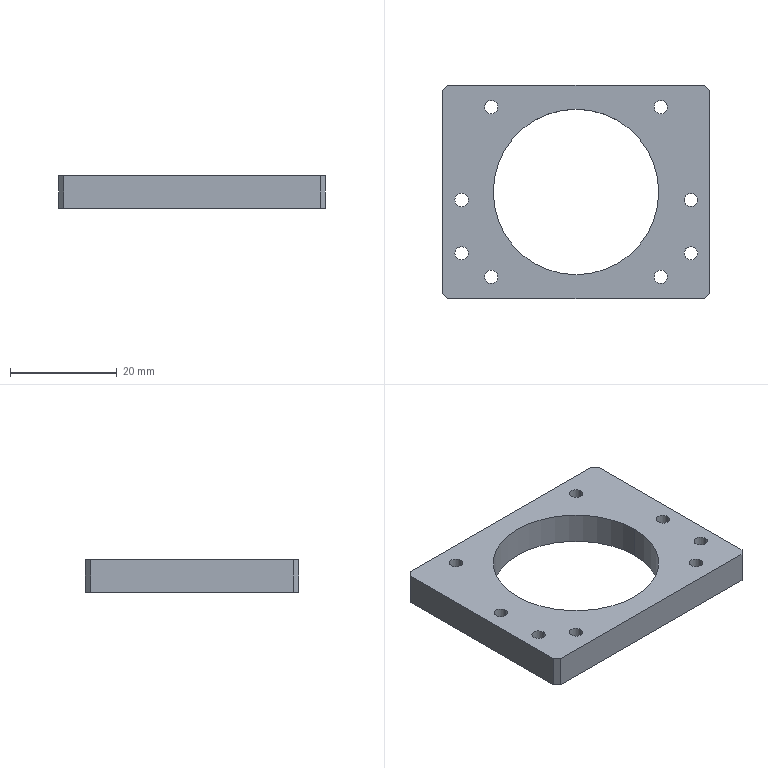Part | NX | features BREP 1 | 1 solid | 28 faces | box 50 x 40 x 6 mm | volume 7224 mm3 | cylinder 18 | plane 10 | commonest cylinder face diameters 2.5 x16 31 x2
STEP:
#1=CARTESIAN_POINT('',(20.3,-11.5,6.));
#2=VERTEX_POINT('',#1);
#3=CARTESIAN_POINT('',(22.8,-11.5,6.));
#4=VERTEX_POINT('',#3);
#5=CARTESIAN_POINT('',(21.55,-11.5,6.));
#6=DIRECTION('',(0.,0.,1.));
#7=DIRECTION('',(1.,0.,0.));
#8=AXIS2_PLACEMENT_3D('',#5,#6,#7);
#9=CIRCLE('',#8,1.25);
#10=EDGE_CURVE('',#2,#4,#9,.T.);
#11=ORIENTED_EDGE('',*,*,#10,.T.);
#12=CARTESIAN_POINT('',(22.8,-11.5,0.));
#13=VERTEX_POINT('',#12);
#14=CARTESIAN_POINT('',(22.8,-11.5,0.));
#15=DIRECTION('',(0.,0.,-1.));
#16=VECTOR('',#15,1000.);
#17=LINE('',#14,#16);
#18=EDGE_CURVE('',#4,#13,#17,.T.);
#19=ORIENTED_EDGE('',*,*,#18,.T.);
#20=CARTESIAN_POINT('',(20.3,-11.5,0.));
#21=VERTEX_POINT('',#20);
#22=CARTESIAN_POINT('',(21.55,-11.5,0.));
#23=DIRECTION('',(0.,0.,-1.));
#24=DIRECTION('',(-1.,0.,0.));
#25=AXIS2_PLACEMENT_3D('',#22,#23,#24);
#26=CIRCLE('',#25,1.25);
#27=EDGE_CURVE('',#13,#21,#26,.T.);
#28=ORIENTED_EDGE('',*,*,#27,.T.);
#29=CARTESIAN_POINT('',(20.3,-11.5,0.));
#30=DIRECTION('',(0.,0.,-1.));
#31=VECTOR('',#30,1000.);
#32=LINE('',#29,#31);
#33=EDGE_CURVE('',#2,#21,#32,.T.);
#34=ORIENTED_EDGE('',*,*,#33,.F.);
#35=EDGE_LOOP('',(#11,#19,#28,#34));
#36=FACE_BOUND('',#35,.T.);
#37=CARTESIAN_POINT('',(21.55,-11.5,0.));
#38=DIRECTION('',(0.,0.,-1.));
#39=DIRECTION('',(-1.,0.,0.));
#40=AXIS2_PLACEMENT_3D('',#37,#38,#39);
#41=CYLINDRICAL_SURFACE('',#40,1.25);
#42=ADVANCED_FACE('',(#36),#41,.F.);
#43=CARTESIAN_POINT('',(-22.7,-11.5,6.));
#44=VERTEX_POINT('',#43);
#45=CARTESIAN_POINT('',(-20.2,-11.5,6.));
#46=VERTEX_POINT('',#45);
#47=CARTESIAN_POINT('',(-21.45,-11.5,6.));
#48=DIRECTION('',(0.,0.,1.));
#49=DIRECTION('',(1.,0.,0.));
#50=AXIS2_PLACEMENT_3D('',#47,#48,#49);
#51=CIRCLE('',#50,1.25);
#52=EDGE_CURVE('',#44,#46,#51,.T.);
#53=ORIENTED_EDGE('',*,*,#52,.T.);
#54=CARTESIAN_POINT('',(-20.2,-11.5,0.));
#55=VERTEX_POINT('',#54);
#56=CARTESIAN_POINT('',(-20.2,-11.5,0.));
#57=DIRECTION('',(0.,0.,-1.));
#58=VECTOR('',#57,1000.);
#59=LINE('',#56,#58);
#60=EDGE_CURVE('',#46,#55,#59,.T.);
#61=ORIENTED_EDGE('',*,*,#60,.T.);
#62=CARTESIAN_POINT('',(-22.7,-11.5,0.));
#63=VERTEX_POINT('',#62);
#64=CARTESIAN_POINT('',(-21.45,-11.5,0.));
#65=DIRECTION('',(0.,0.,-1.));
#66=DIRECTION('',(-1.,0.,0.));
#67=AXIS2_PLACEMENT_3D('',#64,#65,#66);
#68=CIRCLE('',#67,1.25);
#69=EDGE_CURVE('',#55,#63,#68,.T.);
#70=ORIENTED_EDGE('',*,*,#69,.T.);
#71=CARTESIAN_POINT('',(-22.7,-11.5,0.));
#72=DIRECTION('',(0.,0.,-1.));
#73=VECTOR('',#72,1000.);
#74=LINE('',#71,#73);
#75=EDGE_CURVE('',#44,#63,#74,.T.);
#76=ORIENTED_EDGE('',*,*,#75,.F.);
#77=EDGE_LOOP('',(#53,#61,#70,#76));
#78=FACE_BOUND('',#77,.T.);
#79=CARTESIAN_POINT('',(-21.45,-11.5,0.));
#80=DIRECTION('',(0.,0.,-1.));
#81=DIRECTION('',(-1.,0.,0.));
#82=AXIS2_PLACEMENT_3D('',#79,#80,#81);
#83=CYLINDRICAL_SURFACE('',#82,1.25);
#84=ADVANCED_FACE('',(#78),#83,.F.);
#85=CARTESIAN_POINT('',(-22.7,-1.5,6.));
#86=VERTEX_POINT('',#85);
#87=CARTESIAN_POINT('',(-20.2,-1.5,6.));
#88=VERTEX_POINT('',#87);
#89=CARTESIAN_POINT('',(-21.45,-1.5,6.));
#90=DIRECTION('',(0.,0.,1.));
#91=DIRECTION('',(1.,0.,0.));
#92=AXIS2_PLACEMENT_3D('',#89,#90,#91);
#93=CIRCLE('',#92,1.25);
#94=EDGE_CURVE('',#86,#88,#93,.T.);
#95=ORIENTED_EDGE('',*,*,#94,.T.);
#96=CARTESIAN_POINT('',(-20.2,-1.5,0.));
#97=VERTEX_POINT('',#96);
#98=CARTESIAN_POINT('',(-20.2,-1.5,0.));
#99=DIRECTION('',(0.,0.,-1.));
#100=VECTOR('',#99,1000.);
#101=LINE('',#98,#100);
#102=EDGE_CURVE('',#88,#97,#101,.T.);
#103=ORIENTED_EDGE('',*,*,#102,.T.);
#104=CARTESIAN_POINT('',(-22.7,-1.5,0.));
#105=VERTEX_POINT('',#104);
#106=CARTESIAN_POINT('',(-21.45,-1.5,0.));
#107=DIRECTION('',(0.,0.,-1.));
#108=DIRECTION('',(-1.,0.,0.));
#109=AXIS2_PLACEMENT_3D('',#106,#107,#108);
#110=CIRCLE('',#109,1.25);
#111=EDGE_CURVE('',#97,#105,#110,.T.);
#112=ORIENTED_EDGE('',*,*,#111,.T.);
#113=CARTESIAN_POINT('',(-22.7,-1.5,0.));
#114=DIRECTION('',(0.,0.,-1.));
#115=VECTOR('',#114,1000.);
#116=LINE('',#113,#115);
#117=EDGE_CURVE('',#86,#105,#116,.T.);
#118=ORIENTED_EDGE('',*,*,#117,.F.);
#119=EDGE_LOOP('',(#95,#103,#112,#118));
#120=FACE_BOUND('',#119,.T.);
#121=CARTESIAN_POINT('',(-21.45,-1.5,0.));
#122=DIRECTION('',(0.,0.,-1.));
#123=DIRECTION('',(-1.,0.,0.));
#124=AXIS2_PLACEMENT_3D('',#121,#122,#123);
#125=CYLINDRICAL_SURFACE('',#124,1.25);
#126=ADVANCED_FACE('',(#120),#125,.F.);
#127=CARTESIAN_POINT('',(20.3,-1.5,6.));
#128=VERTEX_POINT('',#127);
#129=CARTESIAN_POINT('',(22.8,-1.5,6.));
#130=VERTEX_POINT('',#129);
#131=CARTESIAN_POINT('',(21.55,-1.5,6.));
#132=DIRECTION('',(0.,0.,1.));
#133=DIRECTION('',(1.,0.,0.));
#134=AXIS2_PLACEMENT_3D('',#131,#132,#133);
#135=CIRCLE('',#134,1.25);
#136=EDGE_CURVE('',#128,#130,#135,.T.);
#137=ORIENTED_EDGE('',*,*,#136,.T.);
#138=CARTESIAN_POINT('',(22.8,-1.5,0.));
#139=VERTEX_POINT('',#138);
#140=CARTESIAN_POINT('',(22.8,-1.5,0.));
#141=DIRECTION('',(0.,0.,-1.));
#142=VECTOR('',#141,1000.);
#143=LINE('',#140,#142);
#144=EDGE_CURVE('',#130,#139,#143,.T.);
#145=ORIENTED_EDGE('',*,*,#144,.T.);
#146=CARTESIAN_POINT('',(20.3,-1.5,0.));
#147=VERTEX_POINT('',#146);
#148=CARTESIAN_POINT('',(21.55,-1.5,0.));
#149=DIRECTION('',(0.,0.,-1.));
#150=DIRECTION('',(-1.,0.,0.));
#151=AXIS2_PLACEMENT_3D('',#148,#149,#150);
#152=CIRCLE('',#151,1.25);
#153=EDGE_CURVE('',#139,#147,#152,.T.);
#154=ORIENTED_EDGE('',*,*,#153,.T.);
#155=CARTESIAN_POINT('',(20.3,-1.5,0.));
#156=DIRECTION('',(0.,0.,-1.));
#157=VECTOR('',#156,1000.);
#158=LINE('',#155,#157);
#159=EDGE_CURVE('',#128,#147,#158,.T.);
#160=ORIENTED_EDGE('',*,*,#159,.F.);
#161=EDGE_LOOP('',(#137,#145,#154,#160));
#162=FACE_BOUND('',#161,.T.);
#163=CARTESIAN_POINT('',(21.55,-1.5,0.));
#164=DIRECTION('',(0.,0.,-1.));
#165=DIRECTION('',(-1.,0.,0.));
#166=AXIS2_PLACEMENT_3D('',#163,#164,#165);
#167=CYLINDRICAL_SURFACE('',#166,1.25);
#168=ADVANCED_FACE('',(#162),#167,.F.);
#169=CARTESIAN_POINT('',(17.16,15.91,6.));
#170=VERTEX_POINT('',#169);
#171=CARTESIAN_POINT('',(14.66,15.91,6.));
#172=VERTEX_POINT('',#171);
#173=CARTESIAN_POINT('',(15.91,15.91,6.));
#174=DIRECTION('',(0.,0.,-1.));
#175=DIRECTION('',(-1.,0.,0.));
#176=AXIS2_PLACEMENT_3D('',#173,#174,#175);
#177=CIRCLE('',#176,1.25);
#178=EDGE_CURVE('',#170,#172,#177,.T.);
#179=ORIENTED_EDGE('',*,*,#178,.F.);
#180=CARTESIAN_POINT('',(17.16,15.91,0.));
#181=VERTEX_POINT('',#180);
#182=CARTESIAN_POINT('',(17.16,15.91,0.));
#183=DIRECTION('',(0.,0.,-1.));
#184=VECTOR('',#183,1000.);
#185=LINE('',#182,#184);
#186=EDGE_CURVE('',#170,#181,#185,.T.);
#187=ORIENTED_EDGE('',*,*,#186,.T.);
#188=CARTESIAN_POINT('',(14.66,15.91,0.));
#189=VERTEX_POINT('',#188);
#190=CARTESIAN_POINT('',(15.91,15.91,0.));
#191=DIRECTION('',(0.,0.,-1.));
#192=DIRECTION('',(-1.,0.,0.));
#193=AXIS2_PLACEMENT_3D('',#190,#191,#192);
#194=CIRCLE('',#193,1.25);
#195=EDGE_CURVE('',#181,#189,#194,.T.);
#196=ORIENTED_EDGE('',*,*,#195,.T.);
#197=CARTESIAN_POINT('',(14.66,15.91,0.));
#198=DIRECTION('',(0.,0.,-1.));
#199=VECTOR('',#198,1000.);
#200=LINE('',#197,#199);
#201=EDGE_CURVE('',#172,#189,#200,.T.);
#202=ORIENTED_EDGE('',*,*,#201,.F.);
#203=EDGE_LOOP('',(#179,#187,#196,#202));
#204=FACE_BOUND('',#203,.T.);
#205=CARTESIAN_POINT('',(15.91,15.91,0.));
#206=DIRECTION('',(0.,0.,-1.));
#207=DIRECTION('',(-1.,0.,0.));
#208=AXIS2_PLACEMENT_3D('',#205,#206,#207);
#209=CYLINDRICAL_SURFACE('',#208,1.25);
#210=ADVANCED_FACE('',(#204),#209,.F.);
#211=CARTESIAN_POINT('',(-14.66,15.91,6.));
#212=VERTEX_POINT('',#211);
#213=CARTESIAN_POINT('',(-17.16,15.91,6.));
#214=VERTEX_POINT('',#213);
#215=CARTESIAN_POINT('',(-15.91,15.91,6.));
#216=DIRECTION('',(0.,0.,-1.));
#217=DIRECTION('',(-1.,0.,0.));
#218=AXIS2_PLACEMENT_3D('',#215,#216,#217);
#219=CIRCLE('',#218,1.25);
#220=EDGE_CURVE('',#212,#214,#219,.T.);
#221=ORIENTED_EDGE('',*,*,#220,.F.);
#222=CARTESIAN_POINT('',(-14.66,15.91,0.));
#223=VERTEX_POINT('',#222);
#224=CARTESIAN_POINT('',(-14.66,15.91,0.));
#225=DIRECTION('',(0.,0.,-1.));
#226=VECTOR('',#225,1000.);
#227=LINE('',#224,#226);
#228=EDGE_CURVE('',#212,#223,#227,.T.);
#229=ORIENTED_EDGE('',*,*,#228,.T.);
#230=CARTESIAN_POINT('',(-17.16,15.91,0.));
#231=VERTEX_POINT('',#230);
#232=CARTESIAN_POINT('',(-15.91,15.91,0.));
#233=DIRECTION('',(0.,0.,-1.));
#234=DIRECTION('',(-1.,0.,0.));
#235=AXIS2_PLACEMENT_3D('',#232,#233,#234);
#236=CIRCLE('',#235,1.25);
#237=EDGE_CURVE('',#223,#231,#236,.T.);
#238=ORIENTED_EDGE('',*,*,#237,.T.);
#239=CARTESIAN_POINT('',(-17.16,15.91,0.));
#240=DIRECTION('',(0.,0.,-1.));
#241=VECTOR('',#240,1000.);
#242=LINE('',#239,#241);
#243=EDGE_CURVE('',#214,#231,#242,.T.);
#244=ORIENTED_EDGE('',*,*,#243,.F.);
#245=EDGE_LOOP('',(#221,#229,#238,#244));
#246=FACE_BOUND('',#245,.T.);
#247=CARTESIAN_POINT('',(-15.91,15.91,0.));
#248=DIRECTION('',(0.,0.,-1.));
#249=DIRECTION('',(-1.,0.,0.));
#250=AXIS2_PLACEMENT_3D('',#247,#248,#249);
#251=CYLINDRICAL_SURFACE('',#250,1.25);
#252=ADVANCED_FACE('',(#246),#251,.F.);
#253=CARTESIAN_POINT('',(-14.66,-15.91,6.));
#254=VERTEX_POINT('',#253);
#255=CARTESIAN_POINT('',(-17.16,-15.91,6.));
#256=VERTEX_POINT('',#255);
#257=CARTESIAN_POINT('',(-15.91,-15.91,6.));
#258=DIRECTION('',(0.,0.,-1.));
#259=DIRECTION('',(-1.,0.,0.));
#260=AXIS2_PLACEMENT_3D('',#257,#258,#259);
#261=CIRCLE('',#260,1.25);
#262=EDGE_CURVE('',#254,#256,#261,.T.);
#263=ORIENTED_EDGE('',*,*,#262,.F.);
#264=CARTESIAN_POINT('',(-14.66,-15.91,0.));
#265=VERTEX_POINT('',#264);
#266=CARTESIAN_POINT('',(-14.66,-15.91,0.));
#267=DIRECTION('',(0.,0.,-1.));
#268=VECTOR('',#267,1000.);
#269=LINE('',#266,#268);
#270=EDGE_CURVE('',#254,#265,#269,.T.);
#271=ORIENTED_EDGE('',*,*,#270,.T.);
#272=CARTESIAN_POINT('',(-17.16,-15.91,0.));
#273=VERTEX_POINT('',#272);
#274=CARTESIAN_POINT('',(-15.91,-15.91,0.));
#275=DIRECTION('',(0.,0.,-1.));
#276=DIRECTION('',(-1.,0.,0.));
#277=AXIS2_PLACEMENT_3D('',#274,#275,#276);
#278=CIRCLE('',#277,1.25);
#279=EDGE_CURVE('',#265,#273,#278,.T.);
#280=ORIENTED_EDGE('',*,*,#279,.T.);
#281=CARTESIAN_POINT('',(-17.16,-15.91,0.));
#282=DIRECTION('',(0.,0.,-1.));
#283=VECTOR('',#282,1000.);
#284=LINE('',#281,#283);
#285=EDGE_CURVE('',#256,#273,#284,.T.);
#286=ORIENTED_EDGE('',*,*,#285,.F.);
#287=EDGE_LOOP('',(#263,#271,#280,#286));
#288=FACE_BOUND('',#287,.T.);
#289=CARTESIAN_POINT('',(-15.91,-15.91,0.));
#290=DIRECTION('',(0.,0.,-1.));
#291=DIRECTION('',(-1.,0.,0.));
#292=AXIS2_PLACEMENT_3D('',#289,#290,#291);
#293=CYLINDRICAL_SURFACE('',#292,1.25);
#294=ADVANCED_FACE('',(#288),#293,.F.);
#295=CARTESIAN_POINT('',(17.16,-15.91,6.));
#296=VERTEX_POINT('',#295);
#297=CARTESIAN_POINT('',(14.66,-15.91,6.));
#298=VERTEX_POINT('',#297);
#299=CARTESIAN_POINT('',(15.91,-15.91,6.));
#300=DIRECTION('',(0.,0.,-1.));
#301=DIRECTION('',(-1.,0.,0.));
#302=AXIS2_PLACEMENT_3D('',#299,#300,#301);
#303=CIRCLE('',#302,1.25);
#304=EDGE_CURVE('',#296,#298,#303,.T.);
#305=ORIENTED_EDGE('',*,*,#304,.F.);
#306=CARTESIAN_POINT('',(17.16,-15.91,0.));
#307=VERTEX_POINT('',#306);
#308=CARTESIAN_POINT('',(17.16,-15.91,0.));
#309=DIRECTION('',(0.,0.,-1.));
#310=VECTOR('',#309,1000.);
#311=LINE('',#308,#310);
#312=EDGE_CURVE('',#296,#307,#311,.T.);
#313=ORIENTED_EDGE('',*,*,#312,.T.);
#314=CARTESIAN_POINT('',(14.66,-15.91,0.));
#315=VERTEX_POINT('',#314);
#316=CARTESIAN_POINT('',(15.91,-15.91,0.));
#317=DIRECTION('',(0.,0.,-1.));
#318=DIRECTION('',(-1.,0.,0.));
#319=AXIS2_PLACEMENT_3D('',#316,#317,#318);
#320=CIRCLE('',#319,1.25);
#321=EDGE_CURVE('',#307,#315,#320,.T.);
#322=ORIENTED_EDGE('',*,*,#321,.T.);
#323=CARTESIAN_POINT('',(14.66,-15.91,0.));
#324=DIRECTION('',(0.,0.,-1.));
#325=VECTOR('',#324,1000.);
#326=LINE('',#323,#325);
#327=EDGE_CURVE('',#298,#315,#326,.T.);
#328=ORIENTED_EDGE('',*,*,#327,.F.);
#329=EDGE_LOOP('',(#305,#313,#322,#328));
#330=FACE_BOUND('',#329,.T.);
#331=CARTESIAN_POINT('',(15.91,-15.91,0.));
#332=DIRECTION('',(0.,0.,-1.));
#333=DIRECTION('',(-1.,0.,0.));
#334=AXIS2_PLACEMENT_3D('',#331,#332,#333);
#335=CYLINDRICAL_SURFACE('',#334,1.25);
#336=ADVANCED_FACE('',(#330),#335,.F.);
#337=CARTESIAN_POINT('',(-15.5,0.,0.));
#338=VERTEX_POINT('',#337);
#339=CARTESIAN_POINT('',(15.5,0.,0.));
#340=VERTEX_POINT('',#339);
#341=CARTESIAN_POINT('',(0.,0.,0.));
#342=DIRECTION('',(0.,0.,1.));
#343=DIRECTION('',(1.,0.,0.));
#344=AXIS2_PLACEMENT_3D('',#341,#342,#343);
#345=CIRCLE('',#344,15.5);
#346=EDGE_CURVE('',#338,#340,#345,.T.);
#347=ORIENTED_EDGE('',*,*,#346,.F.);
#348=CARTESIAN_POINT('',(-15.5,0.,6.));
#349=VERTEX_POINT('',#348);
#350=CARTESIAN_POINT('',(-15.5,0.,-22.));
#351=DIRECTION('',(0.,0.,1.));
#352=VECTOR('',#351,1000.);
#353=LINE('',#350,#352);
#354=EDGE_CURVE('',#349,#338,#353,.F.);
#355=ORIENTED_EDGE('',*,*,#354,.F.);
#356=CARTESIAN_POINT('',(15.5,0.,6.));
#357=VERTEX_POINT('',#356);
#358=CARTESIAN_POINT('',(0.,0.,6.));
#359=DIRECTION('',(0.,0.,1.));
#360=DIRECTION('',(1.,0.,0.));
#361=AXIS2_PLACEMENT_3D('',#358,#359,#360);
#362=CIRCLE('',#361,15.5);
#363=EDGE_CURVE('',#349,#357,#362,.T.);
#364=ORIENTED_EDGE('',*,*,#363,.T.);
#365=CARTESIAN_POINT('',(15.5,0.,-22.));
#366=DIRECTION('',(0.,0.,1.));
#367=VECTOR('',#366,1000.);
#368=LINE('',#365,#367);
#369=EDGE_CURVE('',#357,#340,#368,.F.);
#370=ORIENTED_EDGE('',*,*,#369,.T.);
#371=EDGE_LOOP('',(#347,#355,#364,#370));
#372=FACE_BOUND('',#371,.T.);
#373=CARTESIAN_POINT('',(0.,0.,-22.));
#374=DIRECTION('',(0.,0.,1.));
#375=DIRECTION('',(1.,0.,0.));
#376=AXIS2_PLACEMENT_3D('',#373,#374,#375);
#377=CYLINDRICAL_SURFACE('',#376,15.5);
#378=ADVANCED_FACE('',(#372),#377,.F.);
#379=CARTESIAN_POINT('',(25.,-19.,6.));
#380=VERTEX_POINT('',#379);
#381=CARTESIAN_POINT('',(25.,19.,6.));
#382=VERTEX_POINT('',#381);
#383=CARTESIAN_POINT('',(25.,20.,6.));
#384=DIRECTION('',(0.,1.,0.));
#385=VECTOR('',#384,1000.);
#386=LINE('',#383,#385);
#387=EDGE_CURVE('',#380,#382,#386,.T.);
#388=ORIENTED_EDGE('',*,*,#387,.F.);
#389=CARTESIAN_POINT('',(25.,-19.,0.));
#390=VERTEX_POINT('',#389);
#391=CARTESIAN_POINT('',(25.,-19.,6.));
#392=DIRECTION('',(0.,0.,-1.));
#393=VECTOR('',#392,1000.);
#394=LINE('',#391,#393);
#395=EDGE_CURVE('',#380,#390,#394,.T.);
#396=ORIENTED_EDGE('',*,*,#395,.T.);
#397=CARTESIAN_POINT('',(25.,19.,0.));
#398=VERTEX_POINT('',#397);
#399=CARTESIAN_POINT('',(25.,20.,0.));
#400=DIRECTION('',(0.,1.,0.));
#401=VECTOR('',#400,1000.);
#402=LINE('',#399,#401);
#403=EDGE_CURVE('',#390,#398,#402,.T.);
#404=ORIENTED_EDGE('',*,*,#403,.T.);
#405=CARTESIAN_POINT('',(25.,19.,6.));
#406=DIRECTION('',(0.,0.,1.));
#407=VECTOR('',#406,1000.);
#408=LINE('',#405,#407);
#409=EDGE_CURVE('',#398,#382,#408,.T.);
#410=ORIENTED_EDGE('',*,*,#409,.T.);
#411=EDGE_LOOP('',(#388,#396,#404,#410));
#412=FACE_BOUND('',#411,.T.);
#413=CARTESIAN_POINT('',(25.,20.,6.));
#414=DIRECTION('',(-1.,0.,0.));
#415=DIRECTION('',(0.,1.,0.));
#416=AXIS2_PLACEMENT_3D('',#413,#414,#415);
#417=PLANE('',#416);
#418=ADVANCED_FACE('',(#412),#417,.F.);
#419=CARTESIAN_POINT('',(24.,20.,6.));
#420=VERTEX_POINT('',#419);
#421=CARTESIAN_POINT('',(-24.,20.,6.));
#422=VERTEX_POINT('',#421);
#423=CARTESIAN_POINT('',(-25.,20.,6.));
#424=DIRECTION('',(-1.,0.,0.));
#425=VECTOR('',#424,1000.);
#426=LINE('',#423,#425);
#427=EDGE_CURVE('',#420,#422,#426,.T.);
#428=ORIENTED_EDGE('',*,*,#427,.F.);
#429=CARTESIAN_POINT('',(24.,20.,0.));
#430=VERTEX_POINT('',#429);
#431=CARTESIAN_POINT('',(24.,20.,6.));
#432=DIRECTION('',(0.,0.,-1.));
#433=VECTOR('',#432,1000.);
#434=LINE('',#431,#433);
#435=EDGE_CURVE('',#420,#430,#434,.T.);
#436=ORIENTED_EDGE('',*,*,#435,.T.);
#437=CARTESIAN_POINT('',(-24.,20.,0.));
#438=VERTEX_POINT('',#437);
#439=CARTESIAN_POINT('',(-25.,20.,0.));
#440=DIRECTION('',(-1.,0.,0.));
#441=VECTOR('',#440,1000.);
#442=LINE('',#439,#441);
#443=EDGE_CURVE('',#430,#438,#442,.T.);
#444=ORIENTED_EDGE('',*,*,#443,.T.);
#445=CARTESIAN_POINT('',(-24.,20.,6.));
#446=DIRECTION('',(0.,0.,1.));
#447=VECTOR('',#446,1000.);
#448=LINE('',#445,#447);
#449=EDGE_CURVE('',#438,#422,#448,.T.);
#450=ORIENTED_EDGE('',*,*,#449,.T.);
#451=EDGE_LOOP('',(#428,#436,#444,#450));
#452=FACE_BOUND('',#451,.T.);
#453=CARTESIAN_POINT('',(-25.,20.,6.));
#454=DIRECTION('',(0.,-1.,0.));
#455=DIRECTION('',(0.,0.,-1.));
#456=AXIS2_PLACEMENT_3D('',#453,#454,#455);
#457=PLANE('',#456);
#458=ADVANCED_FACE('',(#452),#457,.F.);
#459=CARTESIAN_POINT('',(-25.,19.,0.));
#460=VERTEX_POINT('',#459);
#461=CARTESIAN_POINT('',(-25.,-19.,0.));
#462=VERTEX_POINT('',#461);
#463=CARTESIAN_POINT('',(-25.,20.,0.));
#464=DIRECTION('',(0.,-1.,0.));
#465=VECTOR('',#464,1000.);
#466=LINE('',#463,#465);
#467=EDGE_CURVE('',#460,#462,#466,.T.);
#468=ORIENTED_EDGE('',*,*,#467,.T.);
#469=CARTESIAN_POINT('',(-25.,-19.,6.));
#470=VERTEX_POINT('',#469);
#471=CARTESIAN_POINT('',(-25.,-19.,6.));
#472=DIRECTION('',(0.,0.,1.));
#473=VECTOR('',#472,1000.);
#474=LINE('',#471,#473);
#475=EDGE_CURVE('',#462,#470,#474,.T.);
#476=ORIENTED_EDGE('',*,*,#475,.T.);
#477=CARTESIAN_POINT('',(-25.,19.,6.));
#478=VERTEX_POINT('',#477);
#479=CARTESIAN_POINT('',(-25.,20.,6.));
#480=DIRECTION('',(0.,-1.,0.));
#481=VECTOR('',#480,1000.);
#482=LINE('',#479,#481);
#483=EDGE_CURVE('',#478,#470,#482,.T.);
#484=ORIENTED_EDGE('',*,*,#483,.F.);
#485=CARTESIAN_POINT('',(-25.,19.,6.));
#486=DIRECTION('',(0.,0.,-1.));
#487=VECTOR('',#486,1000.);
#488=LINE('',#485,#487);
#489=EDGE_CURVE('',#478,#460,#488,.T.);
#490=ORIENTED_EDGE('',*,*,#489,.T.);
#491=EDGE_LOOP('',(#468,#476,#484,#490));
#492=FACE_BOUND('',#491,.T.);
#493=CARTESIAN_POINT('',(-25.,20.,6.));
#494=DIRECTION('',(1.,0.,0.));
#495=DIRECTION('',(0.,1.,0.));
#496=AXIS2_PLACEMENT_3D('',#493,#494,#495);
#497=PLANE('',#496);
#498=ADVANCED_FACE('',(#492),#497,.F.);
#499=CARTESIAN_POINT('',(-24.,-20.,6.));
#500=VERTEX_POINT('',#499);
#501=CARTESIAN_POINT('',(24.,-20.,6.));
#502=VERTEX_POINT('',#501);
#503=CARTESIAN_POINT('',(-25.,-20.,6.));
#504=DIRECTION('',(1.,0.,0.));
#505=VECTOR('',#504,1000.);
#506=LINE('',#503,#505);
#507=EDGE_CURVE('',#500,#502,#506,.T.);
#508=ORIENTED_EDGE('',*,*,#507,.F.);
#509=CARTESIAN_POINT('',(-24.,-20.,0.));
#510=VERTEX_POINT('',#509);
#511=CARTESIAN_POINT('',(-24.,-20.,6.));
#512=DIRECTION('',(0.,0.,-1.));
#513=VECTOR('',#512,1000.);
#514=LINE('',#511,#513);
#515=EDGE_CURVE('',#500,#510,#514,.T.);
#516=ORIENTED_EDGE('',*,*,#515,.T.);
#517=CARTESIAN_POINT('',(24.,-20.,0.));
#518=VERTEX_POINT('',#517);
#519=CARTESIAN_POINT('',(-25.,-20.,0.));
#520=DIRECTION('',(1.,0.,0.));
#521=VECTOR('',#520,1000.);
#522=LINE('',#519,#521);
#523=EDGE_CURVE('',#510,#518,#522,.T.);
#524=ORIENTED_EDGE('',*,*,#523,.T.);
#525=CARTESIAN_POINT('',(24.,-20.,6.));
#526=DIRECTION('',(0.,0.,1.));
#527=VECTOR('',#526,1000.);
#528=LINE('',#525,#527);
#529=EDGE_CURVE('',#518,#502,#528,.T.);
#530=ORIENTED_EDGE('',*,*,#529,.T.);
#531=EDGE_LOOP('',(#508,#516,#524,#530));
#532=FACE_BOUND('',#531,.T.);
#533=CARTESIAN_POINT('',(-25.,-20.,6.));
#534=DIRECTION('',(0.,1.,0.));
#535=DIRECTION('',(1.,0.,0.));
#536=AXIS2_PLACEMENT_3D('',#533,#534,#535);
#537=PLANE('',#536);
#538=ADVANCED_FACE('',(#532),#537,.F.);
#539=ORIENTED_EDGE('',*,*,#483,.T.);
#540=CARTESIAN_POINT('',(-22.,-22.,6.));
#541=DIRECTION('',(0.7071,-0.7071,0.));
#542=VECTOR('',#541,1000.);
#543=LINE('',#540,#542);
#544=EDGE_CURVE('',#470,#500,#543,.T.);
#545=ORIENTED_EDGE('',*,*,#544,.T.);
#546=ORIENTED_EDGE('',*,*,#507,.T.);
#547=CARTESIAN_POINT('',(22.,-22.,6.));
#548=DIRECTION('',(0.7071,0.7071,0.));
#549=VECTOR('',#548,1000.);
#550=LINE('',#547,#549);
#551=EDGE_CURVE('',#502,#380,#550,.T.);
#552=ORIENTED_EDGE('',*,*,#551,.T.);
#553=ORIENTED_EDGE('',*,*,#387,.T.);
#554=CARTESIAN_POINT('',(22.,22.,6.));
#555=DIRECTION('',(-0.7071,0.7071,0.));
#556=VECTOR('',#555,1000.);
#557=LINE('',#554,#556);
#558=EDGE_CURVE('',#382,#420,#557,.T.);
#559=ORIENTED_EDGE('',*,*,#558,.T.);
#560=ORIENTED_EDGE('',*,*,#427,.T.);
#561=CARTESIAN_POINT('',(-22.,22.,6.));
#562=DIRECTION('',(-0.7071,-0.7071,0.));
#563=VECTOR('',#562,1000.);
#564=LINE('',#561,#563);
#565=EDGE_CURVE('',#422,#478,#564,.T.);
#566=ORIENTED_EDGE('',*,*,#565,.T.);
#567=EDGE_LOOP('',(#539,#545,#546,#552,#553,#559,#560,#566));
#568=FACE_BOUND('',#567,.T.);
#569=ORIENTED_EDGE('',*,*,#10,.F.);
#570=CARTESIAN_POINT('',(21.55,-11.5,6.));
#571=DIRECTION('',(0.,0.,1.));
#572=DIRECTION('',(1.,0.,0.));
#573=AXIS2_PLACEMENT_3D('',#570,#571,#572);
#574=CIRCLE('',#573,1.25);
#575=EDGE_CURVE('',#4,#2,#574,.T.);
#576=ORIENTED_EDGE('',*,*,#575,.F.);
#577=EDGE_LOOP('',(#569,#576));
#578=FACE_BOUND('',#577,.T.);
#579=ORIENTED_EDGE('',*,*,#52,.F.);
#580=CARTESIAN_POINT('',(-21.45,-11.5,6.));
#581=DIRECTION('',(0.,0.,1.));
#582=DIRECTION('',(1.,0.,0.));
#583=AXIS2_PLACEMENT_3D('',#580,#581,#582);
#584=CIRCLE('',#583,1.25);
#585=EDGE_CURVE('',#46,#44,#584,.T.);
#586=ORIENTED_EDGE('',*,*,#585,.F.);
#587=EDGE_LOOP('',(#579,#586));
#588=FACE_BOUND('',#587,.T.);
#589=ORIENTED_EDGE('',*,*,#94,.F.);
#590=CARTESIAN_POINT('',(-21.45,-1.5,6.));
#591=DIRECTION('',(0.,0.,1.));
#592=DIRECTION('',(1.,0.,0.));
#593=AXIS2_PLACEMENT_3D('',#590,#591,#592);
#594=CIRCLE('',#593,1.25);
#595=EDGE_CURVE('',#88,#86,#594,.T.);
#596=ORIENTED_EDGE('',*,*,#595,.F.);
#597=EDGE_LOOP('',(#589,#596));
#598=FACE_BOUND('',#597,.T.);
#599=ORIENTED_EDGE('',*,*,#136,.F.);
#600=CARTESIAN_POINT('',(21.55,-1.5,6.));
#601=DIRECTION('',(0.,0.,1.));
#602=DIRECTION('',(1.,0.,0.));
#603=AXIS2_PLACEMENT_3D('',#600,#601,#602);
#604=CIRCLE('',#603,1.25);
#605=EDGE_CURVE('',#130,#128,#604,.T.);
#606=ORIENTED_EDGE('',*,*,#605,.F.);
#607=EDGE_LOOP('',(#599,#606));
#608=FACE_BOUND('',#607,.T.);
#609=CARTESIAN_POINT('',(15.91,15.91,6.));
#610=DIRECTION('',(0.,0.,-1.));
#611=DIRECTION('',(-1.,0.,0.));
#612=AXIS2_PLACEMENT_3D('',#609,#610,#611);
#613=CIRCLE('',#612,1.25);
#614=EDGE_CURVE('',#172,#170,#613,.T.);
#615=ORIENTED_EDGE('',*,*,#614,.T.);
#616=ORIENTED_EDGE('',*,*,#178,.T.);
#617=EDGE_LOOP('',(#615,#616));
#618=FACE_BOUND('',#617,.T.);
#619=CARTESIAN_POINT('',(-15.91,15.91,6.));
#620=DIRECTION('',(0.,0.,-1.));
#621=DIRECTION('',(-1.,0.,0.));
#622=AXIS2_PLACEMENT_3D('',#619,#620,#621);
#623=CIRCLE('',#622,1.25);
#624=EDGE_CURVE('',#214,#212,#623,.T.);
#625=ORIENTED_EDGE('',*,*,#624,.T.);
#626=ORIENTED_EDGE('',*,*,#220,.T.);
#627=EDGE_LOOP('',(#625,#626));
#628=FACE_BOUND('',#627,.T.);
#629=CARTESIAN_POINT('',(-15.91,-15.91,6.));
#630=DIRECTION('',(0.,0.,-1.));
#631=DIRECTION('',(-1.,0.,0.));
#632=AXIS2_PLACEMENT_3D('',#629,#630,#631);
#633=CIRCLE('',#632,1.25);
#634=EDGE_CURVE('',#256,#254,#633,.T.);
#635=ORIENTED_EDGE('',*,*,#634,.T.);
#636=ORIENTED_EDGE('',*,*,#262,.T.);
#637=EDGE_LOOP('',(#635,#636));
#638=FACE_BOUND('',#637,.T.);
#639=CARTESIAN_POINT('',(15.91,-15.91,6.));
#640=DIRECTION('',(0.,0.,-1.));
#641=DIRECTION('',(-1.,0.,0.));
#642=AXIS2_PLACEMENT_3D('',#639,#640,#641);
#643=CIRCLE('',#642,1.25);
#644=EDGE_CURVE('',#298,#296,#643,.T.);
#645=ORIENTED_EDGE('',*,*,#644,.T.);
#646=ORIENTED_EDGE('',*,*,#304,.T.);
#647=EDGE_LOOP('',(#645,#646));
#648=FACE_BOUND('',#647,.T.);
#649=CARTESIAN_POINT('',(0.,0.,6.));
#650=DIRECTION('',(0.,0.,1.));
#651=DIRECTION('',(1.,0.,0.));
#652=AXIS2_PLACEMENT_3D('',#649,#650,#651);
#653=CIRCLE('',#652,15.5);
#654=EDGE_CURVE('',#357,#349,#653,.T.);
#655=ORIENTED_EDGE('',*,*,#654,.F.);
#656=ORIENTED_EDGE('',*,*,#363,.F.);
#657=EDGE_LOOP('',(#655,#656));
#658=FACE_BOUND('',#657,.T.);
#659=CARTESIAN_POINT('',(0.,0.,6.));
#660=DIRECTION('',(0.,0.,1.));
#661=DIRECTION('',(1.,0.,0.));
#662=AXIS2_PLACEMENT_3D('',#659,#660,#661);
#663=PLANE('',#662);
#664=ADVANCED_FACE('',(#568,#578,#588,#598,#608,#618,#628,#638,#648,#658),#663,.T.);
#665=ORIENTED_EDGE('',*,*,#523,.F.);
#666=CARTESIAN_POINT('',(-24.,-20.,0.));
#667=DIRECTION('',(-0.7071,0.7071,0.));
#668=VECTOR('',#667,1000.);
#669=LINE('',#666,#668);
#670=EDGE_CURVE('',#510,#462,#669,.T.);
#671=ORIENTED_EDGE('',*,*,#670,.T.);
#672=ORIENTED_EDGE('',*,*,#467,.F.);
#673=CARTESIAN_POINT('',(-25.,19.,0.));
#674=DIRECTION('',(0.7071,0.7071,0.));
#675=VECTOR('',#674,1000.);
#676=LINE('',#673,#675);
#677=EDGE_CURVE('',#460,#438,#676,.T.);
#678=ORIENTED_EDGE('',*,*,#677,.T.);
#679=ORIENTED_EDGE('',*,*,#443,.F.);
#680=CARTESIAN_POINT('',(24.,20.,0.));
#681=DIRECTION('',(0.7071,-0.7071,0.));
#682=VECTOR('',#681,1000.);
#683=LINE('',#680,#682);
#684=EDGE_CURVE('',#430,#398,#683,.T.);
#685=ORIENTED_EDGE('',*,*,#684,.T.);
#686=ORIENTED_EDGE('',*,*,#403,.F.);
#687=CARTESIAN_POINT('',(25.,-19.,0.));
#688=DIRECTION('',(-0.7071,-0.7071,0.));
#689=VECTOR('',#688,1000.);
#690=LINE('',#687,#689);
#691=EDGE_CURVE('',#390,#518,#690,.T.);
#692=ORIENTED_EDGE('',*,*,#691,.T.);
#693=EDGE_LOOP('',(#665,#671,#672,#678,#679,#685,#686,#692));
#694=FACE_BOUND('',#693,.T.);
#695=CARTESIAN_POINT('',(21.55,-11.5,0.));
#696=DIRECTION('',(0.,0.,-1.));
#697=DIRECTION('',(-1.,0.,0.));
#698=AXIS2_PLACEMENT_3D('',#695,#696,#697);
#699=CIRCLE('',#698,1.25);
#700=EDGE_CURVE('',#21,#13,#699,.T.);
#701=ORIENTED_EDGE('',*,*,#700,.F.);
#702=ORIENTED_EDGE('',*,*,#27,.F.);
#703=EDGE_LOOP('',(#701,#702));
#704=FACE_BOUND('',#703,.T.);
#705=CARTESIAN_POINT('',(-21.45,-11.5,0.));
#706=DIRECTION('',(0.,0.,-1.));
#707=DIRECTION('',(-1.,0.,0.));
#708=AXIS2_PLACEMENT_3D('',#705,#706,#707);
#709=CIRCLE('',#708,1.25);
#710=EDGE_CURVE('',#63,#55,#709,.T.);
#711=ORIENTED_EDGE('',*,*,#710,.F.);
#712=ORIENTED_EDGE('',*,*,#69,.F.);
#713=EDGE_LOOP('',(#711,#712));
#714=FACE_BOUND('',#713,.T.);
#715=CARTESIAN_POINT('',(-21.45,-1.5,0.));
#716=DIRECTION('',(0.,0.,-1.));
#717=DIRECTION('',(-1.,0.,0.));
#718=AXIS2_PLACEMENT_3D('',#715,#716,#717);
#719=CIRCLE('',#718,1.25);
#720=EDGE_CURVE('',#105,#97,#719,.T.);
#721=ORIENTED_EDGE('',*,*,#720,.F.);
#722=ORIENTED_EDGE('',*,*,#111,.F.);
#723=EDGE_LOOP('',(#721,#722));
#724=FACE_BOUND('',#723,.T.);
#725=CARTESIAN_POINT('',(21.55,-1.5,0.));
#726=DIRECTION('',(0.,0.,-1.));
#727=DIRECTION('',(-1.,0.,0.));
#728=AXIS2_PLACEMENT_3D('',#725,#726,#727);
#729=CIRCLE('',#728,1.25);
#730=EDGE_CURVE('',#147,#139,#729,.T.);
#731=ORIENTED_EDGE('',*,*,#730,.F.);
#732=ORIENTED_EDGE('',*,*,#153,.F.);
#733=EDGE_LOOP('',(#731,#732));
#734=FACE_BOUND('',#733,.T.);
#735=CARTESIAN_POINT('',(15.91,15.91,0.));
#736=DIRECTION('',(0.,0.,-1.));
#737=DIRECTION('',(-1.,0.,0.));
#738=AXIS2_PLACEMENT_3D('',#735,#736,#737);
#739=CIRCLE('',#738,1.25);
#740=EDGE_CURVE('',#189,#181,#739,.T.);
#741=ORIENTED_EDGE('',*,*,#740,.F.);
#742=ORIENTED_EDGE('',*,*,#195,.F.);
#743=EDGE_LOOP('',(#741,#742));
#744=FACE_BOUND('',#743,.T.);
#745=CARTESIAN_POINT('',(-15.91,15.91,0.));
#746=DIRECTION('',(0.,0.,-1.));
#747=DIRECTION('',(-1.,0.,0.));
#748=AXIS2_PLACEMENT_3D('',#745,#746,#747);
#749=CIRCLE('',#748,1.25);
#750=EDGE_CURVE('',#231,#223,#749,.T.);
#751=ORIENTED_EDGE('',*,*,#750,.F.);
#752=ORIENTED_EDGE('',*,*,#237,.F.);
#753=EDGE_LOOP('',(#751,#752));
#754=FACE_BOUND('',#753,.T.);
#755=CARTESIAN_POINT('',(-15.91,-15.91,0.));
#756=DIRECTION('',(0.,0.,-1.));
#757=DIRECTION('',(-1.,0.,0.));
#758=AXIS2_PLACEMENT_3D('',#755,#756,#757);
#759=CIRCLE('',#758,1.25);
#760=EDGE_CURVE('',#273,#265,#759,.T.);
#761=ORIENTED_EDGE('',*,*,#760,.F.);
#762=ORIENTED_EDGE('',*,*,#279,.F.);
#763=EDGE_LOOP('',(#761,#762));
#764=FACE_BOUND('',#763,.T.);
#765=CARTESIAN_POINT('',(15.91,-15.91,0.));
#766=DIRECTION('',(0.,0.,-1.));
#767=DIRECTION('',(-1.,0.,0.));
#768=AXIS2_PLACEMENT_3D('',#765,#766,#767);
#769=CIRCLE('',#768,1.25);
#770=EDGE_CURVE('',#315,#307,#769,.T.);
#771=ORIENTED_EDGE('',*,*,#770,.F.);
#772=ORIENTED_EDGE('',*,*,#321,.F.);
#773=EDGE_LOOP('',(#771,#772));
#774=FACE_BOUND('',#773,.T.);
#775=CARTESIAN_POINT('',(0.,0.,0.));
#776=DIRECTION('',(0.,0.,1.));
#777=DIRECTION('',(1.,0.,0.));
#778=AXIS2_PLACEMENT_3D('',#775,#776,#777);
#779=CIRCLE('',#778,15.5);
#780=EDGE_CURVE('',#340,#338,#779,.T.);
#781=ORIENTED_EDGE('',*,*,#780,.T.);
#782=ORIENTED_EDGE('',*,*,#346,.T.);
#783=EDGE_LOOP('',(#781,#782));
#784=FACE_BOUND('',#783,.T.);
#785=CARTESIAN_POINT('',(0.,0.,0.));
#786=DIRECTION('',(0.,0.,1.));
#787=DIRECTION('',(1.,0.,0.));
#788=AXIS2_PLACEMENT_3D('',#785,#786,#787);
#789=PLANE('',#788);
#790=ADVANCED_FACE('',(#694,#704,#714,#724,#734,#744,#754,#764,#774,#784),#789,.F.);
#791=ORIENTED_EDGE('',*,*,#354,.T.);
#792=ORIENTED_EDGE('',*,*,#780,.F.);
#793=ORIENTED_EDGE('',*,*,#369,.F.);
#794=ORIENTED_EDGE('',*,*,#654,.T.);
#795=EDGE_LOOP('',(#791,#792,#793,#794));
#796=FACE_BOUND('',#795,.T.);
#797=CARTESIAN_POINT('',(0.,0.,-22.));
#798=DIRECTION('',(0.,0.,1.));
#799=DIRECTION('',(1.,0.,0.));
#800=AXIS2_PLACEMENT_3D('',#797,#798,#799);
#801=CYLINDRICAL_SURFACE('',#800,15.5);
#802=ADVANCED_FACE('',(#796),#801,.F.);
#803=ORIENTED_EDGE('',*,*,#544,.F.);
#804=ORIENTED_EDGE('',*,*,#475,.F.);
#805=ORIENTED_EDGE('',*,*,#670,.F.);
#806=ORIENTED_EDGE('',*,*,#515,.F.);
#807=EDGE_LOOP('',(#803,#804,#805,#806));
#808=FACE_BOUND('',#807,.T.);
#809=CARTESIAN_POINT('',(-24.,-20.,6.));
#810=DIRECTION('',(0.7071,0.7071,0.));
#811=DIRECTION('',(0.,0.,-1.));
#812=AXIS2_PLACEMENT_3D('',#809,#810,#811);
#813=PLANE('',#812);
#814=ADVANCED_FACE('',(#808),#813,.F.);
#815=ORIENTED_EDGE('',*,*,#551,.F.);
#816=ORIENTED_EDGE('',*,*,#529,.F.);
#817=ORIENTED_EDGE('',*,*,#691,.F.);
#818=ORIENTED_EDGE('',*,*,#395,.F.);
#819=EDGE_LOOP('',(#815,#816,#817,#818));
#820=FACE_BOUND('',#819,.T.);
#821=CARTESIAN_POINT('',(25.,-19.,6.));
#822=DIRECTION('',(-0.7071,0.7071,0.));
#823=DIRECTION('',(0.,0.,1.));
#824=AXIS2_PLACEMENT_3D('',#821,#822,#823);
#825=PLANE('',#824);
#826=ADVANCED_FACE('',(#820),#825,.F.);
#827=ORIENTED_EDGE('',*,*,#558,.F.);
#828=ORIENTED_EDGE('',*,*,#409,.F.);
#829=ORIENTED_EDGE('',*,*,#684,.F.);
#830=ORIENTED_EDGE('',*,*,#435,.F.);
#831=EDGE_LOOP('',(#827,#828,#829,#830));
#832=FACE_BOUND('',#831,.T.);
#833=CARTESIAN_POINT('',(24.,20.,6.));
#834=DIRECTION('',(-0.7071,-0.7071,0.));
#835=DIRECTION('',(-0.7071,0.7071,0.));
#836=AXIS2_PLACEMENT_3D('',#833,#834,#835);
#837=PLANE('',#836);
#838=ADVANCED_FACE('',(#832),#837,.F.);
#839=ORIENTED_EDGE('',*,*,#565,.F.);
#840=ORIENTED_EDGE('',*,*,#449,.F.);
#841=ORIENTED_EDGE('',*,*,#677,.F.);
#842=ORIENTED_EDGE('',*,*,#489,.F.);
#843=EDGE_LOOP('',(#839,#840,#841,#842));
#844=FACE_BOUND('',#843,.T.);
#845=CARTESIAN_POINT('',(-25.,19.,6.));
#846=DIRECTION('',(0.7071,-0.7071,0.));
#847=DIRECTION('',(0.,0.,-1.));
#848=AXIS2_PLACEMENT_3D('',#845,#846,#847);
#849=PLANE('',#848);
#850=ADVANCED_FACE('',(#844),#849,.F.);
#851=ORIENTED_EDGE('',*,*,#312,.F.);
#852=ORIENTED_EDGE('',*,*,#644,.F.);
#853=ORIENTED_EDGE('',*,*,#327,.T.);
#854=ORIENTED_EDGE('',*,*,#770,.T.);
#855=EDGE_LOOP('',(#851,#852,#853,#854));
#856=FACE_BOUND('',#855,.T.);
#857=CARTESIAN_POINT('',(15.91,-15.91,0.));
#858=DIRECTION('',(0.,0.,-1.));
#859=DIRECTION('',(-1.,0.,0.));
#860=AXIS2_PLACEMENT_3D('',#857,#858,#859);
#861=CYLINDRICAL_SURFACE('',#860,1.25);
#862=ADVANCED_FACE('',(#856),#861,.F.);
#863=ORIENTED_EDGE('',*,*,#270,.F.);
#864=ORIENTED_EDGE('',*,*,#634,.F.);
#865=ORIENTED_EDGE('',*,*,#285,.T.);
#866=ORIENTED_EDGE('',*,*,#760,.T.);
#867=EDGE_LOOP('',(#863,#864,#865,#866));
#868=FACE_BOUND('',#867,.T.);
#869=CARTESIAN_POINT('',(-15.91,-15.91,0.));
#870=DIRECTION('',(0.,0.,-1.));
#871=DIRECTION('',(-1.,0.,0.));
#872=AXIS2_PLACEMENT_3D('',#869,#870,#871);
#873=CYLINDRICAL_SURFACE('',#872,1.25);
#874=ADVANCED_FACE('',(#868),#873,.F.);
#875=ORIENTED_EDGE('',*,*,#228,.F.);
#876=ORIENTED_EDGE('',*,*,#624,.F.);
#877=ORIENTED_EDGE('',*,*,#243,.T.);
#878=ORIENTED_EDGE('',*,*,#750,.T.);
#879=EDGE_LOOP('',(#875,#876,#877,#878));
#880=FACE_BOUND('',#879,.T.);
#881=CARTESIAN_POINT('',(-15.91,15.91,0.));
#882=DIRECTION('',(0.,0.,-1.));
#883=DIRECTION('',(-1.,0.,0.));
#884=AXIS2_PLACEMENT_3D('',#881,#882,#883);
#885=CYLINDRICAL_SURFACE('',#884,1.25);
#886=ADVANCED_FACE('',(#880),#885,.F.);
#887=ORIENTED_EDGE('',*,*,#186,.F.);
#888=ORIENTED_EDGE('',*,*,#614,.F.);
#889=ORIENTED_EDGE('',*,*,#201,.T.);
#890=ORIENTED_EDGE('',*,*,#740,.T.);
#891=EDGE_LOOP('',(#887,#888,#889,#890));
#892=FACE_BOUND('',#891,.T.);
#893=CARTESIAN_POINT('',(15.91,15.91,0.));
#894=DIRECTION('',(0.,0.,-1.));
#895=DIRECTION('',(-1.,0.,0.));
#896=AXIS2_PLACEMENT_3D('',#893,#894,#895);
#897=CYLINDRICAL_SURFACE('',#896,1.25);
#898=ADVANCED_FACE('',(#892),#897,.F.);
#899=ORIENTED_EDGE('',*,*,#144,.F.);
#900=ORIENTED_EDGE('',*,*,#605,.T.);
#901=ORIENTED_EDGE('',*,*,#159,.T.);
#902=ORIENTED_EDGE('',*,*,#730,.T.);
#903=EDGE_LOOP('',(#899,#900,#901,#902));
#904=FACE_BOUND('',#903,.T.);
#905=CARTESIAN_POINT('',(21.55,-1.5,0.));
#906=DIRECTION('',(0.,0.,-1.));
#907=DIRECTION('',(-1.,0.,0.));
#908=AXIS2_PLACEMENT_3D('',#905,#906,#907);
#909=CYLINDRICAL_SURFACE('',#908,1.25);
#910=ADVANCED_FACE('',(#904),#909,.F.);
#911=ORIENTED_EDGE('',*,*,#102,.F.);
#912=ORIENTED_EDGE('',*,*,#595,.T.);
#913=ORIENTED_EDGE('',*,*,#117,.T.);
#914=ORIENTED_EDGE('',*,*,#720,.T.);
#915=EDGE_LOOP('',(#911,#912,#913,#914));
#916=FACE_BOUND('',#915,.T.);
#917=CARTESIAN_POINT('',(-21.45,-1.5,0.));
#918=DIRECTION('',(0.,0.,-1.));
#919=DIRECTION('',(-1.,0.,0.));
#920=AXIS2_PLACEMENT_3D('',#917,#918,#919);
#921=CYLINDRICAL_SURFACE('',#920,1.25);
#922=ADVANCED_FACE('',(#916),#921,.F.);
#923=ORIENTED_EDGE('',*,*,#60,.F.);
#924=ORIENTED_EDGE('',*,*,#585,.T.);
#925=ORIENTED_EDGE('',*,*,#75,.T.);
#926=ORIENTED_EDGE('',*,*,#710,.T.);
#927=EDGE_LOOP('',(#923,#924,#925,#926));
#928=FACE_BOUND('',#927,.T.);
#929=CARTESIAN_POINT('',(-21.45,-11.5,0.));
#930=DIRECTION('',(0.,0.,-1.));
#931=DIRECTION('',(-1.,0.,0.));
#932=AXIS2_PLACEMENT_3D('',#929,#930,#931);
#933=CYLINDRICAL_SURFACE('',#932,1.25);
#934=ADVANCED_FACE('',(#928),#933,.F.);
#935=ORIENTED_EDGE('',*,*,#18,.F.);
#936=ORIENTED_EDGE('',*,*,#575,.T.);
#937=ORIENTED_EDGE('',*,*,#33,.T.);
#938=ORIENTED_EDGE('',*,*,#700,.T.);
#939=EDGE_LOOP('',(#935,#936,#937,#938));
#940=FACE_BOUND('',#939,.T.);
#941=CARTESIAN_POINT('',(21.55,-11.5,0.));
#942=DIRECTION('',(0.,0.,-1.));
#943=DIRECTION('',(-1.,0.,0.));
#944=AXIS2_PLACEMENT_3D('',#941,#942,#943);
#945=CYLINDRICAL_SURFACE('',#944,1.25);
#946=ADVANCED_FACE('',(#940),#945,.F.);
#947=CLOSED_SHELL('',(#42,#84,#126,#168,#210,#252,#294,#336,#378,#418,#458,#498,#538,#664,#790,#802,#814,#826,#838,#850,#862,#874,#886,#898,#910,#922,#934,#946));
#948=MANIFOLD_SOLID_BREP('',#947);
#949=(LENGTH_UNIT()NAMED_UNIT(*)SI_UNIT(.MILLI.,.METRE.));
#950=UNCERTAINTY_MEASURE_WITH_UNIT(LENGTH_MEASURE(0.00001),#949,'','');
#951=(NAMED_UNIT(*)PLANE_ANGLE_UNIT()SI_UNIT($,.RADIAN.));
#952=(NAMED_UNIT(*)SI_UNIT($,.STERADIAN.)SOLID_ANGLE_UNIT());
#953=(GEOMETRIC_REPRESENTATION_CONTEXT(3)GLOBAL_UNCERTAINTY_ASSIGNED_CONTEXT((#950))GLOBAL_UNIT_ASSIGNED_CONTEXT((#949,#951,#952))REPRESENTATION_CONTEXT('',''));
#954=ADVANCED_BREP_SHAPE_REPRESENTATION('',(#948),#953);